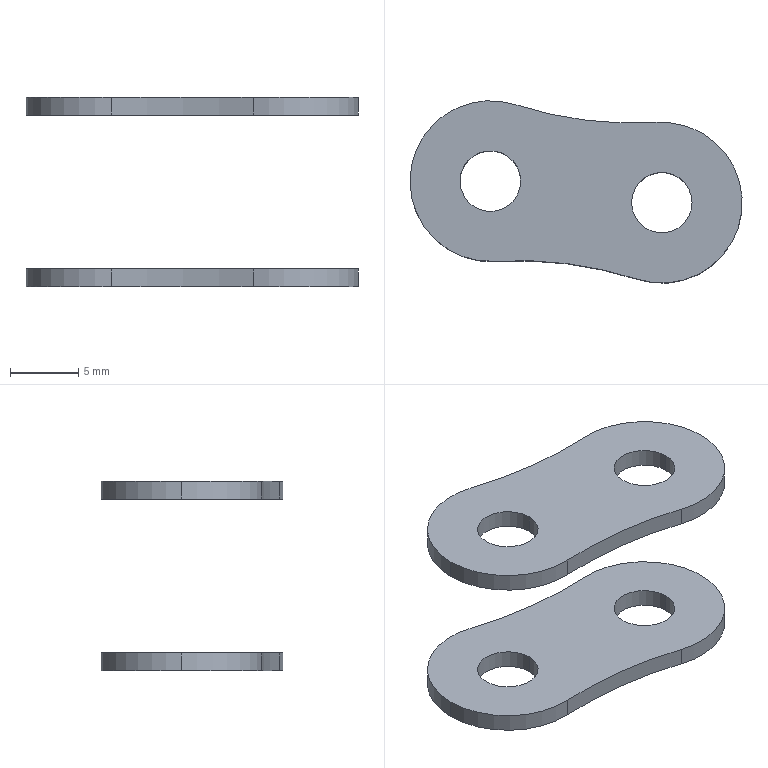Part | SolidWorks | features Boss 2, DeleteBody 1, Extrusion 1, MirrorSolid 1 | 2 solids | 22 faces | box 24.41 x 13.399 x 13.92 mm | volume 574.494 mm3 | cylinder 18 | plane 4 | commonest cylinder face diameters 4.45 x8 11.81 x6 57.066 x4
STEP:
#1=CARTESIAN_POINT('',(16.725,-1.589,6.96));
#2=VERTEX_POINT('',#1);
#3=CARTESIAN_POINT('',(21.175,-1.589,6.96));
#4=VERTEX_POINT('',#3);
#5=CARTESIAN_POINT('',(18.95,-1.589,6.96));
#6=DIRECTION('',(0.,0.,1.));
#7=DIRECTION('',(1.,0.,0.));
#8=AXIS2_PLACEMENT_3D('',#5,#6,#7);
#9=CIRCLE('',#8,2.225);
#10=EDGE_CURVE('',#2,#4,#9,.T.);
#11=ORIENTED_EDGE('',*,*,#10,.T.);
#12=CARTESIAN_POINT('',(21.175,-1.589,5.65));
#13=VERTEX_POINT('',#12);
#14=CARTESIAN_POINT('',(21.175,-1.589,6.96));
#15=DIRECTION('',(0.,0.,-1.));
#16=VECTOR('',#15,1000.);
#17=LINE('',#14,#16);
#18=EDGE_CURVE('',#4,#13,#17,.T.);
#19=ORIENTED_EDGE('',*,*,#18,.T.);
#20=CARTESIAN_POINT('',(16.725,-1.589,5.65));
#21=VERTEX_POINT('',#20);
#22=CARTESIAN_POINT('',(18.95,-1.589,5.65));
#23=DIRECTION('',(0.,0.,1.));
#24=DIRECTION('',(1.,0.,0.));
#25=AXIS2_PLACEMENT_3D('',#22,#23,#24);
#26=CIRCLE('',#25,2.225);
#27=EDGE_CURVE('',#21,#13,#26,.T.);
#28=ORIENTED_EDGE('',*,*,#27,.F.);
#29=CARTESIAN_POINT('',(16.725,-1.589,6.96));
#30=DIRECTION('',(0.,0.,-1.));
#31=VECTOR('',#30,1000.);
#32=LINE('',#29,#31);
#33=EDGE_CURVE('',#2,#21,#32,.T.);
#34=ORIENTED_EDGE('',*,*,#33,.F.);
#35=EDGE_LOOP('',(#11,#19,#28,#34));
#36=FACE_OUTER_BOUND('',#35,.T.);
#37=CARTESIAN_POINT('',(18.95,-1.589,6.96));
#38=DIRECTION('',(0.,0.,-1.));
#39=DIRECTION('',(-1.,0.,0.));
#40=AXIS2_PLACEMENT_3D('',#37,#38,#39);
#41=CYLINDRICAL_SURFACE('',#40,2.225);
#42=ADVANCED_FACE('',(#36),#41,.F.);
#43=CARTESIAN_POINT('',(4.125,0.,6.96));
#44=VERTEX_POINT('',#43);
#45=CARTESIAN_POINT('',(8.575,0.,6.96));
#46=VERTEX_POINT('',#45);
#47=CARTESIAN_POINT('',(6.35,0.,6.96));
#48=DIRECTION('',(0.,0.,1.));
#49=DIRECTION('',(1.,0.,0.));
#50=AXIS2_PLACEMENT_3D('',#47,#48,#49);
#51=CIRCLE('',#50,2.225);
#52=EDGE_CURVE('',#44,#46,#51,.T.);
#53=ORIENTED_EDGE('',*,*,#52,.T.);
#54=CARTESIAN_POINT('',(8.575,0.,5.65));
#55=VERTEX_POINT('',#54);
#56=CARTESIAN_POINT('',(8.575,0.,6.96));
#57=DIRECTION('',(0.,0.,-1.));
#58=VECTOR('',#57,1000.);
#59=LINE('',#56,#58);
#60=EDGE_CURVE('',#46,#55,#59,.T.);
#61=ORIENTED_EDGE('',*,*,#60,.T.);
#62=CARTESIAN_POINT('',(4.125,0.,5.65));
#63=VERTEX_POINT('',#62);
#64=CARTESIAN_POINT('',(6.35,0.,5.65));
#65=DIRECTION('',(0.,0.,1.));
#66=DIRECTION('',(1.,0.,0.));
#67=AXIS2_PLACEMENT_3D('',#64,#65,#66);
#68=CIRCLE('',#67,2.225);
#69=EDGE_CURVE('',#63,#55,#68,.T.);
#70=ORIENTED_EDGE('',*,*,#69,.F.);
#71=CARTESIAN_POINT('',(4.125,0.,6.96));
#72=DIRECTION('',(0.,0.,-1.));
#73=VECTOR('',#72,1000.);
#74=LINE('',#71,#73);
#75=EDGE_CURVE('',#44,#63,#74,.T.);
#76=ORIENTED_EDGE('',*,*,#75,.F.);
#77=EDGE_LOOP('',(#53,#61,#70,#76));
#78=FACE_OUTER_BOUND('',#77,.T.);
#79=CARTESIAN_POINT('',(6.35,0.,6.96));
#80=DIRECTION('',(0.,0.,-1.));
#81=DIRECTION('',(-1.,0.,0.));
#82=AXIS2_PLACEMENT_3D('',#79,#80,#81);
#83=CYLINDRICAL_SURFACE('',#82,2.225);
#84=ADVANCED_FACE('',(#78),#83,.F.);
#85=CARTESIAN_POINT('',(0.445,0.,6.96));
#86=VERTEX_POINT('',#85);
#87=CARTESIAN_POINT('',(6.704,-5.894,6.96));
#88=VERTEX_POINT('',#87);
#89=CARTESIAN_POINT('',(6.35,0.,6.96));
#90=DIRECTION('',(0.,0.,1.));
#91=DIRECTION('',(1.,0.,0.));
#92=AXIS2_PLACEMENT_3D('',#89,#90,#91);
#93=CIRCLE('',#92,5.905);
#94=EDGE_CURVE('',#86,#88,#93,.T.);
#95=ORIENTED_EDGE('',*,*,#94,.F.);
#96=CARTESIAN_POINT('',(0.445,0.,5.65));
#97=VERTEX_POINT('',#96);
#98=CARTESIAN_POINT('',(0.445,0.,6.96));
#99=DIRECTION('',(0.,0.,-1.));
#100=VECTOR('',#99,1000.);
#101=LINE('',#98,#100);
#102=EDGE_CURVE('',#86,#97,#101,.T.);
#103=ORIENTED_EDGE('',*,*,#102,.T.);
#104=CARTESIAN_POINT('',(6.704,-5.894,5.65));
#105=VERTEX_POINT('',#104);
#106=CARTESIAN_POINT('',(6.35,0.,5.65));
#107=DIRECTION('',(0.,0.,1.));
#108=DIRECTION('',(1.,0.,0.));
#109=AXIS2_PLACEMENT_3D('',#106,#107,#108);
#110=CIRCLE('',#109,5.905);
#111=EDGE_CURVE('',#97,#105,#110,.T.);
#112=ORIENTED_EDGE('',*,*,#111,.T.);
#113=CARTESIAN_POINT('',(6.704,-5.894,6.96));
#114=DIRECTION('',(0.,0.,-1.));
#115=VECTOR('',#114,1000.);
#116=LINE('',#113,#115);
#117=EDGE_CURVE('',#88,#105,#116,.T.);
#118=ORIENTED_EDGE('',*,*,#117,.F.);
#119=EDGE_LOOP('',(#95,#103,#112,#118));
#120=FACE_OUTER_BOUND('',#119,.T.);
#121=CARTESIAN_POINT('',(6.35,0.,6.96));
#122=DIRECTION('',(0.,0.,-1.));
#123=DIRECTION('',(-1.,0.,0.));
#124=AXIS2_PLACEMENT_3D('',#121,#122,#123);
#125=CYLINDRICAL_SURFACE('',#124,5.905);
#126=ADVANCED_FACE('',(#120),#125,.T.);
#127=ORIENTED_EDGE('',*,*,#52,.F.);
#128=CARTESIAN_POINT('',(6.35,0.,6.96));
#129=DIRECTION('',(0.,0.,1.));
#130=DIRECTION('',(1.,0.,0.));
#131=AXIS2_PLACEMENT_3D('',#128,#129,#130);
#132=CIRCLE('',#131,2.225);
#133=EDGE_CURVE('',#46,#44,#132,.T.);
#134=ORIENTED_EDGE('',*,*,#133,.F.);
#135=EDGE_LOOP('',(#127,#134));
#136=FACE_BOUND('',#135,.T.);
#137=CARTESIAN_POINT('',(18.596,4.306,6.96));
#138=VERTEX_POINT('',#137);
#139=CARTESIAN_POINT('',(8.156,5.622,6.96));
#140=VERTEX_POINT('',#139);
#141=CARTESIAN_POINT('',(16.884,32.787,6.96));
#142=DIRECTION('',(0.,0.,-1.));
#143=DIRECTION('',(1.,0.,0.));
#144=AXIS2_PLACEMENT_3D('',#141,#142,#143);
#145=CIRCLE('',#144,28.533);
#146=EDGE_CURVE('',#138,#140,#145,.T.);
#147=ORIENTED_EDGE('',*,*,#146,.T.);
#148=CARTESIAN_POINT('',(6.35,0.,6.96));
#149=DIRECTION('',(0.,0.,1.));
#150=DIRECTION('',(1.,0.,0.));
#151=AXIS2_PLACEMENT_3D('',#148,#149,#150);
#152=CIRCLE('',#151,5.905);
#153=EDGE_CURVE('',#140,#86,#152,.T.);
#154=ORIENTED_EDGE('',*,*,#153,.T.);
#155=ORIENTED_EDGE('',*,*,#94,.T.);
#156=CARTESIAN_POINT('',(17.144,-7.211,6.96));
#157=VERTEX_POINT('',#156);
#158=CARTESIAN_POINT('',(8.416,-34.376,6.96));
#159=DIRECTION('',(0.,0.,-1.));
#160=DIRECTION('',(-1.,0.,0.));
#161=AXIS2_PLACEMENT_3D('',#158,#159,#160);
#162=CIRCLE('',#161,28.533);
#163=EDGE_CURVE('',#88,#157,#162,.T.);
#164=ORIENTED_EDGE('',*,*,#163,.T.);
#165=CARTESIAN_POINT('',(18.95,-1.589,6.96));
#166=DIRECTION('',(0.,0.,1.));
#167=DIRECTION('',(1.,0.,0.));
#168=AXIS2_PLACEMENT_3D('',#165,#166,#167);
#169=CIRCLE('',#168,5.905);
#170=EDGE_CURVE('',#157,#138,#169,.T.);
#171=ORIENTED_EDGE('',*,*,#170,.T.);
#172=EDGE_LOOP('',(#147,#154,#155,#164,#171));
#173=FACE_OUTER_BOUND('',#172,.T.);
#174=ORIENTED_EDGE('',*,*,#10,.F.);
#175=CARTESIAN_POINT('',(18.95,-1.589,6.96));
#176=DIRECTION('',(0.,0.,1.));
#177=DIRECTION('',(1.,0.,0.));
#178=AXIS2_PLACEMENT_3D('',#175,#176,#177);
#179=CIRCLE('',#178,2.225);
#180=EDGE_CURVE('',#4,#2,#179,.T.);
#181=ORIENTED_EDGE('',*,*,#180,.F.);
#182=EDGE_LOOP('',(#174,#181));
#183=FACE_BOUND('',#182,.T.);
#184=CARTESIAN_POINT('',(17.917,15.599,6.96));
#185=DIRECTION('',(0.,0.,1.));
#186=DIRECTION('',(1.,0.,0.));
#187=AXIS2_PLACEMENT_3D('',#184,#185,#186);
#188=PLANE('',#187);
#189=ADVANCED_FACE('',(#136,#173,#183),#188,.T.);
#190=CARTESIAN_POINT('',(18.596,4.306,5.65));
#191=VERTEX_POINT('',#190);
#192=CARTESIAN_POINT('',(8.156,5.622,5.65));
#193=VERTEX_POINT('',#192);
#194=CARTESIAN_POINT('',(16.884,32.787,5.65));
#195=DIRECTION('',(0.,0.,-1.));
#196=DIRECTION('',(1.,0.,0.));
#197=AXIS2_PLACEMENT_3D('',#194,#195,#196);
#198=CIRCLE('',#197,28.533);
#199=EDGE_CURVE('',#191,#193,#198,.T.);
#200=ORIENTED_EDGE('',*,*,#199,.F.);
#201=CARTESIAN_POINT('',(17.144,-7.211,5.65));
#202=VERTEX_POINT('',#201);
#203=CARTESIAN_POINT('',(18.95,-1.589,5.65));
#204=DIRECTION('',(0.,0.,1.));
#205=DIRECTION('',(1.,0.,0.));
#206=AXIS2_PLACEMENT_3D('',#203,#204,#205);
#207=CIRCLE('',#206,5.905);
#208=EDGE_CURVE('',#202,#191,#207,.T.);
#209=ORIENTED_EDGE('',*,*,#208,.F.);
#210=CARTESIAN_POINT('',(8.416,-34.376,5.65));
#211=DIRECTION('',(0.,0.,-1.));
#212=DIRECTION('',(-1.,0.,0.));
#213=AXIS2_PLACEMENT_3D('',#210,#211,#212);
#214=CIRCLE('',#213,28.533);
#215=EDGE_CURVE('',#105,#202,#214,.T.);
#216=ORIENTED_EDGE('',*,*,#215,.F.);
#217=ORIENTED_EDGE('',*,*,#111,.F.);
#218=CARTESIAN_POINT('',(6.35,0.,5.65));
#219=DIRECTION('',(0.,0.,1.));
#220=DIRECTION('',(1.,0.,0.));
#221=AXIS2_PLACEMENT_3D('',#218,#219,#220);
#222=CIRCLE('',#221,5.905);
#223=EDGE_CURVE('',#193,#97,#222,.T.);
#224=ORIENTED_EDGE('',*,*,#223,.F.);
#225=EDGE_LOOP('',(#200,#209,#216,#217,#224));
#226=FACE_OUTER_BOUND('',#225,.T.);
#227=ORIENTED_EDGE('',*,*,#69,.T.);
#228=CARTESIAN_POINT('',(6.35,0.,5.65));
#229=DIRECTION('',(0.,0.,1.));
#230=DIRECTION('',(1.,0.,0.));
#231=AXIS2_PLACEMENT_3D('',#228,#229,#230);
#232=CIRCLE('',#231,2.225);
#233=EDGE_CURVE('',#55,#63,#232,.T.);
#234=ORIENTED_EDGE('',*,*,#233,.T.);
#235=EDGE_LOOP('',(#227,#234));
#236=FACE_BOUND('',#235,.T.);
#237=ORIENTED_EDGE('',*,*,#27,.T.);
#238=CARTESIAN_POINT('',(18.95,-1.589,5.65));
#239=DIRECTION('',(0.,0.,1.));
#240=DIRECTION('',(1.,0.,0.));
#241=AXIS2_PLACEMENT_3D('',#238,#239,#240);
#242=CIRCLE('',#241,2.225);
#243=EDGE_CURVE('',#13,#21,#242,.T.);
#244=ORIENTED_EDGE('',*,*,#243,.T.);
#245=EDGE_LOOP('',(#237,#244));
#246=FACE_BOUND('',#245,.T.);
#247=CARTESIAN_POINT('',(17.917,15.599,5.65));
#248=DIRECTION('',(0.,0.,1.));
#249=DIRECTION('',(1.,0.,0.));
#250=AXIS2_PLACEMENT_3D('',#247,#248,#249);
#251=PLANE('',#250);
#252=ADVANCED_FACE('',(#226,#236,#246),#251,.F.);
#253=ORIENTED_EDGE('',*,*,#199,.T.);
#254=CARTESIAN_POINT('',(8.156,5.622,6.96));
#255=DIRECTION('',(0.,0.,-1.));
#256=VECTOR('',#255,1000.);
#257=LINE('',#254,#256);
#258=EDGE_CURVE('',#140,#193,#257,.T.);
#259=ORIENTED_EDGE('',*,*,#258,.F.);
#260=ORIENTED_EDGE('',*,*,#146,.F.);
#261=CARTESIAN_POINT('',(18.596,4.306,6.96));
#262=DIRECTION('',(0.,0.,-1.));
#263=VECTOR('',#262,1000.);
#264=LINE('',#261,#263);
#265=EDGE_CURVE('',#138,#191,#264,.T.);
#266=ORIENTED_EDGE('',*,*,#265,.T.);
#267=EDGE_LOOP('',(#253,#259,#260,#266));
#268=FACE_OUTER_BOUND('',#267,.T.);
#269=CARTESIAN_POINT('',(16.884,32.787,6.96));
#270=DIRECTION('',(0.,0.,-1.));
#271=DIRECTION('',(-1.,0.,0.));
#272=AXIS2_PLACEMENT_3D('',#269,#270,#271);
#273=CYLINDRICAL_SURFACE('',#272,28.533);
#274=ADVANCED_FACE('',(#268),#273,.F.);
#275=ORIENTED_EDGE('',*,*,#102,.F.);
#276=ORIENTED_EDGE('',*,*,#153,.F.);
#277=ORIENTED_EDGE('',*,*,#258,.T.);
#278=ORIENTED_EDGE('',*,*,#223,.T.);
#279=EDGE_LOOP('',(#275,#276,#277,#278));
#280=FACE_OUTER_BOUND('',#279,.T.);
#281=CARTESIAN_POINT('',(6.35,0.,6.96));
#282=DIRECTION('',(0.,0.,-1.));
#283=DIRECTION('',(-1.,0.,0.));
#284=AXIS2_PLACEMENT_3D('',#281,#282,#283);
#285=CYLINDRICAL_SURFACE('',#284,5.905);
#286=ADVANCED_FACE('',(#280),#285,.T.);
#287=ORIENTED_EDGE('',*,*,#215,.T.);
#288=CARTESIAN_POINT('',(17.144,-7.211,6.96));
#289=DIRECTION('',(0.,0.,-1.));
#290=VECTOR('',#289,1000.);
#291=LINE('',#288,#290);
#292=EDGE_CURVE('',#157,#202,#291,.T.);
#293=ORIENTED_EDGE('',*,*,#292,.F.);
#294=ORIENTED_EDGE('',*,*,#163,.F.);
#295=ORIENTED_EDGE('',*,*,#117,.T.);
#296=EDGE_LOOP('',(#287,#293,#294,#295));
#297=FACE_OUTER_BOUND('',#296,.T.);
#298=CARTESIAN_POINT('',(8.416,-34.376,6.96));
#299=DIRECTION('',(0.,0.,-1.));
#300=DIRECTION('',(-1.,0.,0.));
#301=AXIS2_PLACEMENT_3D('',#298,#299,#300);
#302=CYLINDRICAL_SURFACE('',#301,28.533);
#303=ADVANCED_FACE('',(#297),#302,.F.);
#304=ORIENTED_EDGE('',*,*,#208,.T.);
#305=ORIENTED_EDGE('',*,*,#265,.F.);
#306=ORIENTED_EDGE('',*,*,#170,.F.);
#307=ORIENTED_EDGE('',*,*,#292,.T.);
#308=EDGE_LOOP('',(#304,#305,#306,#307));
#309=FACE_OUTER_BOUND('',#308,.T.);
#310=CARTESIAN_POINT('',(18.95,-1.589,6.96));
#311=DIRECTION('',(0.,0.,-1.));
#312=DIRECTION('',(-1.,0.,0.));
#313=AXIS2_PLACEMENT_3D('',#310,#311,#312);
#314=CYLINDRICAL_SURFACE('',#313,5.905);
#315=ADVANCED_FACE('',(#309),#314,.T.);
#316=ORIENTED_EDGE('',*,*,#60,.F.);
#317=ORIENTED_EDGE('',*,*,#133,.T.);
#318=ORIENTED_EDGE('',*,*,#75,.T.);
#319=ORIENTED_EDGE('',*,*,#233,.F.);
#320=EDGE_LOOP('',(#316,#317,#318,#319));
#321=FACE_OUTER_BOUND('',#320,.T.);
#322=CARTESIAN_POINT('',(6.35,0.,6.96));
#323=DIRECTION('',(0.,0.,-1.));
#324=DIRECTION('',(-1.,0.,0.));
#325=AXIS2_PLACEMENT_3D('',#322,#323,#324);
#326=CYLINDRICAL_SURFACE('',#325,2.225);
#327=ADVANCED_FACE('',(#321),#326,.F.);
#328=ORIENTED_EDGE('',*,*,#18,.F.);
#329=ORIENTED_EDGE('',*,*,#180,.T.);
#330=ORIENTED_EDGE('',*,*,#33,.T.);
#331=ORIENTED_EDGE('',*,*,#243,.F.);
#332=EDGE_LOOP('',(#328,#329,#330,#331));
#333=FACE_OUTER_BOUND('',#332,.T.);
#334=CARTESIAN_POINT('',(18.95,-1.589,6.96));
#335=DIRECTION('',(0.,0.,-1.));
#336=DIRECTION('',(-1.,0.,0.));
#337=AXIS2_PLACEMENT_3D('',#334,#335,#336);
#338=CYLINDRICAL_SURFACE('',#337,2.225);
#339=ADVANCED_FACE('',(#333),#338,.F.);
#340=CLOSED_SHELL('',(#42,#84,#126,#189,#252,#274,#286,#303,#315,#327,#339));
#341=MANIFOLD_SOLID_BREP('',#340);
#342=CARTESIAN_POINT('',(21.175,-1.589,-6.96));
#343=VERTEX_POINT('',#342);
#344=CARTESIAN_POINT('',(16.725,-1.589,-6.96));
#345=VERTEX_POINT('',#344);
#346=CARTESIAN_POINT('',(18.95,-1.589,-6.96));
#347=DIRECTION('',(0.,0.,1.));
#348=DIRECTION('',(1.,0.,0.));
#349=AXIS2_PLACEMENT_3D('',#346,#347,#348);
#350=CIRCLE('',#349,2.225);
#351=EDGE_CURVE('',#343,#345,#350,.T.);
#352=ORIENTED_EDGE('',*,*,#351,.F.);
#353=CARTESIAN_POINT('',(21.175,-1.589,-5.65));
#354=VERTEX_POINT('',#353);
#355=CARTESIAN_POINT('',(21.175,-1.589,-6.96));
#356=DIRECTION('',(0.,0.,1.));
#357=VECTOR('',#356,1000.);
#358=LINE('',#355,#357);
#359=EDGE_CURVE('',#343,#354,#358,.T.);
#360=ORIENTED_EDGE('',*,*,#359,.T.);
#361=CARTESIAN_POINT('',(16.725,-1.589,-5.65));
#362=VERTEX_POINT('',#361);
#363=CARTESIAN_POINT('',(18.95,-1.589,-5.65));
#364=DIRECTION('',(0.,0.,1.));
#365=DIRECTION('',(1.,0.,0.));
#366=AXIS2_PLACEMENT_3D('',#363,#364,#365);
#367=CIRCLE('',#366,2.225);
#368=EDGE_CURVE('',#354,#362,#367,.T.);
#369=ORIENTED_EDGE('',*,*,#368,.T.);
#370=CARTESIAN_POINT('',(16.725,-1.589,-6.96));
#371=DIRECTION('',(0.,0.,1.));
#372=VECTOR('',#371,1000.);
#373=LINE('',#370,#372);
#374=EDGE_CURVE('',#345,#362,#373,.T.);
#375=ORIENTED_EDGE('',*,*,#374,.F.);
#376=EDGE_LOOP('',(#352,#360,#369,#375));
#377=FACE_OUTER_BOUND('',#376,.T.);
#378=CARTESIAN_POINT('',(18.95,-1.589,-6.96));
#379=DIRECTION('',(0.,0.,1.));
#380=DIRECTION('',(-1.,0.,0.));
#381=AXIS2_PLACEMENT_3D('',#378,#379,#380);
#382=CYLINDRICAL_SURFACE('',#381,2.225);
#383=ADVANCED_FACE('',(#377),#382,.F.);
#384=CARTESIAN_POINT('',(8.575,0.,-6.96));
#385=VERTEX_POINT('',#384);
#386=CARTESIAN_POINT('',(4.125,0.,-6.96));
#387=VERTEX_POINT('',#386);
#388=CARTESIAN_POINT('',(6.35,0.,-6.96));
#389=DIRECTION('',(0.,0.,1.));
#390=DIRECTION('',(1.,0.,0.));
#391=AXIS2_PLACEMENT_3D('',#388,#389,#390);
#392=CIRCLE('',#391,2.225);
#393=EDGE_CURVE('',#385,#387,#392,.T.);
#394=ORIENTED_EDGE('',*,*,#393,.F.);
#395=CARTESIAN_POINT('',(8.575,0.,-5.65));
#396=VERTEX_POINT('',#395);
#397=CARTESIAN_POINT('',(8.575,0.,-6.96));
#398=DIRECTION('',(0.,0.,1.));
#399=VECTOR('',#398,1000.);
#400=LINE('',#397,#399);
#401=EDGE_CURVE('',#385,#396,#400,.T.);
#402=ORIENTED_EDGE('',*,*,#401,.T.);
#403=CARTESIAN_POINT('',(4.125,0.,-5.65));
#404=VERTEX_POINT('',#403);
#405=CARTESIAN_POINT('',(6.35,0.,-5.65));
#406=DIRECTION('',(0.,0.,1.));
#407=DIRECTION('',(1.,0.,0.));
#408=AXIS2_PLACEMENT_3D('',#405,#406,#407);
#409=CIRCLE('',#408,2.225);
#410=EDGE_CURVE('',#396,#404,#409,.T.);
#411=ORIENTED_EDGE('',*,*,#410,.T.);
#412=CARTESIAN_POINT('',(4.125,0.,-6.96));
#413=DIRECTION('',(0.,0.,1.));
#414=VECTOR('',#413,1000.);
#415=LINE('',#412,#414);
#416=EDGE_CURVE('',#387,#404,#415,.T.);
#417=ORIENTED_EDGE('',*,*,#416,.F.);
#418=EDGE_LOOP('',(#394,#402,#411,#417));
#419=FACE_OUTER_BOUND('',#418,.T.);
#420=CARTESIAN_POINT('',(6.35,0.,-6.96));
#421=DIRECTION('',(0.,0.,1.));
#422=DIRECTION('',(-1.,0.,0.));
#423=AXIS2_PLACEMENT_3D('',#420,#421,#422);
#424=CYLINDRICAL_SURFACE('',#423,2.225);
#425=ADVANCED_FACE('',(#419),#424,.F.);
#426=CARTESIAN_POINT('',(8.156,5.622,-6.96));
#427=VERTEX_POINT('',#426);
#428=CARTESIAN_POINT('',(0.445,0.,-6.96));
#429=VERTEX_POINT('',#428);
#430=CARTESIAN_POINT('',(6.35,0.,-6.96));
#431=DIRECTION('',(0.,0.,1.));
#432=DIRECTION('',(1.,0.,0.));
#433=AXIS2_PLACEMENT_3D('',#430,#431,#432);
#434=CIRCLE('',#433,5.905);
#435=EDGE_CURVE('',#427,#429,#434,.T.);
#436=ORIENTED_EDGE('',*,*,#435,.T.);
#437=CARTESIAN_POINT('',(0.445,0.,-5.65));
#438=VERTEX_POINT('',#437);
#439=CARTESIAN_POINT('',(0.445,0.,-6.96));
#440=DIRECTION('',(0.,0.,1.));
#441=VECTOR('',#440,1000.);
#442=LINE('',#439,#441);
#443=EDGE_CURVE('',#429,#438,#442,.T.);
#444=ORIENTED_EDGE('',*,*,#443,.T.);
#445=CARTESIAN_POINT('',(8.156,5.622,-5.65));
#446=VERTEX_POINT('',#445);
#447=CARTESIAN_POINT('',(6.35,0.,-5.65));
#448=DIRECTION('',(0.,0.,1.));
#449=DIRECTION('',(1.,0.,0.));
#450=AXIS2_PLACEMENT_3D('',#447,#448,#449);
#451=CIRCLE('',#450,5.905);
#452=EDGE_CURVE('',#446,#438,#451,.T.);
#453=ORIENTED_EDGE('',*,*,#452,.F.);
#454=CARTESIAN_POINT('',(8.156,5.622,-6.96));
#455=DIRECTION('',(0.,0.,1.));
#456=VECTOR('',#455,1000.);
#457=LINE('',#454,#456);
#458=EDGE_CURVE('',#427,#446,#457,.T.);
#459=ORIENTED_EDGE('',*,*,#458,.F.);
#460=EDGE_LOOP('',(#436,#444,#453,#459));
#461=FACE_OUTER_BOUND('',#460,.T.);
#462=CARTESIAN_POINT('',(6.35,0.,-6.96));
#463=DIRECTION('',(0.,0.,1.));
#464=DIRECTION('',(-1.,0.,0.));
#465=AXIS2_PLACEMENT_3D('',#462,#463,#464);
#466=CYLINDRICAL_SURFACE('',#465,5.905);
#467=ADVANCED_FACE('',(#461),#466,.T.);
#468=CARTESIAN_POINT('',(6.35,0.,-6.96));
#469=DIRECTION('',(0.,0.,1.));
#470=DIRECTION('',(1.,0.,0.));
#471=AXIS2_PLACEMENT_3D('',#468,#469,#470);
#472=CIRCLE('',#471,2.225);
#473=EDGE_CURVE('',#387,#385,#472,.T.);
#474=ORIENTED_EDGE('',*,*,#473,.T.);
#475=ORIENTED_EDGE('',*,*,#393,.T.);
#476=EDGE_LOOP('',(#474,#475));
#477=FACE_BOUND('',#476,.T.);
#478=CARTESIAN_POINT('',(18.596,4.306,-6.96));
#479=VERTEX_POINT('',#478);
#480=CARTESIAN_POINT('',(16.884,32.787,-6.96));
#481=DIRECTION('',(0.,0.,-1.));
#482=DIRECTION('',(1.,0.,0.));
#483=AXIS2_PLACEMENT_3D('',#480,#481,#482);
#484=CIRCLE('',#483,28.533);
#485=EDGE_CURVE('',#479,#427,#484,.T.);
#486=ORIENTED_EDGE('',*,*,#485,.F.);
#487=CARTESIAN_POINT('',(17.144,-7.211,-6.96));
#488=VERTEX_POINT('',#487);
#489=CARTESIAN_POINT('',(18.95,-1.589,-6.96));
#490=DIRECTION('',(0.,0.,1.));
#491=DIRECTION('',(1.,0.,0.));
#492=AXIS2_PLACEMENT_3D('',#489,#490,#491);
#493=CIRCLE('',#492,5.905);
#494=EDGE_CURVE('',#488,#479,#493,.T.);
#495=ORIENTED_EDGE('',*,*,#494,.F.);
#496=CARTESIAN_POINT('',(6.704,-5.894,-6.96));
#497=VERTEX_POINT('',#496);
#498=CARTESIAN_POINT('',(8.416,-34.376,-6.96));
#499=DIRECTION('',(0.,0.,-1.));
#500=DIRECTION('',(-1.,0.,0.));
#501=AXIS2_PLACEMENT_3D('',#498,#499,#500);
#502=CIRCLE('',#501,28.533);
#503=EDGE_CURVE('',#497,#488,#502,.T.);
#504=ORIENTED_EDGE('',*,*,#503,.F.);
#505=CARTESIAN_POINT('',(6.35,0.,-6.96));
#506=DIRECTION('',(0.,0.,1.));
#507=DIRECTION('',(1.,0.,0.));
#508=AXIS2_PLACEMENT_3D('',#505,#506,#507);
#509=CIRCLE('',#508,5.905);
#510=EDGE_CURVE('',#429,#497,#509,.T.);
#511=ORIENTED_EDGE('',*,*,#510,.F.);
#512=ORIENTED_EDGE('',*,*,#435,.F.);
#513=EDGE_LOOP('',(#486,#495,#504,#511,#512));
#514=FACE_OUTER_BOUND('',#513,.T.);
#515=CARTESIAN_POINT('',(18.95,-1.589,-6.96));
#516=DIRECTION('',(0.,0.,1.));
#517=DIRECTION('',(1.,0.,0.));
#518=AXIS2_PLACEMENT_3D('',#515,#516,#517);
#519=CIRCLE('',#518,2.225);
#520=EDGE_CURVE('',#345,#343,#519,.T.);
#521=ORIENTED_EDGE('',*,*,#520,.T.);
#522=ORIENTED_EDGE('',*,*,#351,.T.);
#523=EDGE_LOOP('',(#521,#522));
#524=FACE_BOUND('',#523,.T.);
#525=CARTESIAN_POINT('',(17.917,15.599,-6.96));
#526=DIRECTION('',(0.,0.,-1.));
#527=DIRECTION('',(1.,0.,0.));
#528=AXIS2_PLACEMENT_3D('',#525,#526,#527);
#529=PLANE('',#528);
#530=ADVANCED_FACE('',(#477,#514,#524),#529,.T.);
#531=CARTESIAN_POINT('',(18.596,4.306,-5.65));
#532=VERTEX_POINT('',#531);
#533=CARTESIAN_POINT('',(16.884,32.787,-5.65));
#534=DIRECTION('',(0.,0.,-1.));
#535=DIRECTION('',(1.,0.,0.));
#536=AXIS2_PLACEMENT_3D('',#533,#534,#535);
#537=CIRCLE('',#536,28.533);
#538=EDGE_CURVE('',#532,#446,#537,.T.);
#539=ORIENTED_EDGE('',*,*,#538,.T.);
#540=ORIENTED_EDGE('',*,*,#452,.T.);
#541=CARTESIAN_POINT('',(6.704,-5.894,-5.65));
#542=VERTEX_POINT('',#541);
#543=CARTESIAN_POINT('',(6.35,0.,-5.65));
#544=DIRECTION('',(0.,0.,1.));
#545=DIRECTION('',(1.,0.,0.));
#546=AXIS2_PLACEMENT_3D('',#543,#544,#545);
#547=CIRCLE('',#546,5.905);
#548=EDGE_CURVE('',#438,#542,#547,.T.);
#549=ORIENTED_EDGE('',*,*,#548,.T.);
#550=CARTESIAN_POINT('',(17.144,-7.211,-5.65));
#551=VERTEX_POINT('',#550);
#552=CARTESIAN_POINT('',(8.416,-34.376,-5.65));
#553=DIRECTION('',(0.,0.,-1.));
#554=DIRECTION('',(-1.,0.,0.));
#555=AXIS2_PLACEMENT_3D('',#552,#553,#554);
#556=CIRCLE('',#555,28.533);
#557=EDGE_CURVE('',#542,#551,#556,.T.);
#558=ORIENTED_EDGE('',*,*,#557,.T.);
#559=CARTESIAN_POINT('',(18.95,-1.589,-5.65));
#560=DIRECTION('',(0.,0.,1.));
#561=DIRECTION('',(1.,0.,0.));
#562=AXIS2_PLACEMENT_3D('',#559,#560,#561);
#563=CIRCLE('',#562,5.905);
#564=EDGE_CURVE('',#551,#532,#563,.T.);
#565=ORIENTED_EDGE('',*,*,#564,.T.);
#566=EDGE_LOOP('',(#539,#540,#549,#558,#565));
#567=FACE_OUTER_BOUND('',#566,.T.);
#568=CARTESIAN_POINT('',(6.35,0.,-5.65));
#569=DIRECTION('',(0.,0.,1.));
#570=DIRECTION('',(1.,0.,0.));
#571=AXIS2_PLACEMENT_3D('',#568,#569,#570);
#572=CIRCLE('',#571,2.225);
#573=EDGE_CURVE('',#404,#396,#572,.T.);
#574=ORIENTED_EDGE('',*,*,#573,.F.);
#575=ORIENTED_EDGE('',*,*,#410,.F.);
#576=EDGE_LOOP('',(#574,#575));
#577=FACE_BOUND('',#576,.T.);
#578=CARTESIAN_POINT('',(18.95,-1.589,-5.65));
#579=DIRECTION('',(0.,0.,1.));
#580=DIRECTION('',(1.,0.,0.));
#581=AXIS2_PLACEMENT_3D('',#578,#579,#580);
#582=CIRCLE('',#581,2.225);
#583=EDGE_CURVE('',#362,#354,#582,.T.);
#584=ORIENTED_EDGE('',*,*,#583,.F.);
#585=ORIENTED_EDGE('',*,*,#368,.F.);
#586=EDGE_LOOP('',(#584,#585));
#587=FACE_BOUND('',#586,.T.);
#588=CARTESIAN_POINT('',(17.917,15.599,-5.65));
#589=DIRECTION('',(0.,0.,-1.));
#590=DIRECTION('',(1.,0.,0.));
#591=AXIS2_PLACEMENT_3D('',#588,#589,#590);
#592=PLANE('',#591);
#593=ADVANCED_FACE('',(#567,#577,#587),#592,.F.);
#594=ORIENTED_EDGE('',*,*,#538,.F.);
#595=CARTESIAN_POINT('',(18.596,4.306,-6.96));
#596=DIRECTION('',(0.,0.,1.));
#597=VECTOR('',#596,1000.);
#598=LINE('',#595,#597);
#599=EDGE_CURVE('',#479,#532,#598,.T.);
#600=ORIENTED_EDGE('',*,*,#599,.F.);
#601=ORIENTED_EDGE('',*,*,#485,.T.);
#602=ORIENTED_EDGE('',*,*,#458,.T.);
#603=EDGE_LOOP('',(#594,#600,#601,#602));
#604=FACE_OUTER_BOUND('',#603,.T.);
#605=CARTESIAN_POINT('',(16.884,32.787,-6.96));
#606=DIRECTION('',(0.,0.,1.));
#607=DIRECTION('',(-1.,0.,0.));
#608=AXIS2_PLACEMENT_3D('',#605,#606,#607);
#609=CYLINDRICAL_SURFACE('',#608,28.533);
#610=ADVANCED_FACE('',(#604),#609,.F.);
#611=ORIENTED_EDGE('',*,*,#443,.F.);
#612=ORIENTED_EDGE('',*,*,#510,.T.);
#613=CARTESIAN_POINT('',(6.704,-5.894,-6.96));
#614=DIRECTION('',(0.,0.,1.));
#615=VECTOR('',#614,1000.);
#616=LINE('',#613,#615);
#617=EDGE_CURVE('',#497,#542,#616,.T.);
#618=ORIENTED_EDGE('',*,*,#617,.T.);
#619=ORIENTED_EDGE('',*,*,#548,.F.);
#620=EDGE_LOOP('',(#611,#612,#618,#619));
#621=FACE_OUTER_BOUND('',#620,.T.);
#622=CARTESIAN_POINT('',(6.35,0.,-6.96));
#623=DIRECTION('',(0.,0.,1.));
#624=DIRECTION('',(-1.,0.,0.));
#625=AXIS2_PLACEMENT_3D('',#622,#623,#624);
#626=CYLINDRICAL_SURFACE('',#625,5.905);
#627=ADVANCED_FACE('',(#621),#626,.T.);
#628=ORIENTED_EDGE('',*,*,#557,.F.);
#629=ORIENTED_EDGE('',*,*,#617,.F.);
#630=ORIENTED_EDGE('',*,*,#503,.T.);
#631=CARTESIAN_POINT('',(17.144,-7.211,-6.96));
#632=DIRECTION('',(0.,0.,1.));
#633=VECTOR('',#632,1000.);
#634=LINE('',#631,#633);
#635=EDGE_CURVE('',#488,#551,#634,.T.);
#636=ORIENTED_EDGE('',*,*,#635,.T.);
#637=EDGE_LOOP('',(#628,#629,#630,#636));
#638=FACE_OUTER_BOUND('',#637,.T.);
#639=CARTESIAN_POINT('',(8.416,-34.376,-6.96));
#640=DIRECTION('',(0.,0.,1.));
#641=DIRECTION('',(-1.,0.,0.));
#642=AXIS2_PLACEMENT_3D('',#639,#640,#641);
#643=CYLINDRICAL_SURFACE('',#642,28.533);
#644=ADVANCED_FACE('',(#638),#643,.F.);
#645=ORIENTED_EDGE('',*,*,#564,.F.);
#646=ORIENTED_EDGE('',*,*,#635,.F.);
#647=ORIENTED_EDGE('',*,*,#494,.T.);
#648=ORIENTED_EDGE('',*,*,#599,.T.);
#649=EDGE_LOOP('',(#645,#646,#647,#648));
#650=FACE_OUTER_BOUND('',#649,.T.);
#651=CARTESIAN_POINT('',(18.95,-1.589,-6.96));
#652=DIRECTION('',(0.,0.,1.));
#653=DIRECTION('',(-1.,0.,0.));
#654=AXIS2_PLACEMENT_3D('',#651,#652,#653);
#655=CYLINDRICAL_SURFACE('',#654,5.905);
#656=ADVANCED_FACE('',(#650),#655,.T.);
#657=ORIENTED_EDGE('',*,*,#401,.F.);
#658=ORIENTED_EDGE('',*,*,#473,.F.);
#659=ORIENTED_EDGE('',*,*,#416,.T.);
#660=ORIENTED_EDGE('',*,*,#573,.T.);
#661=EDGE_LOOP('',(#657,#658,#659,#660));
#662=FACE_OUTER_BOUND('',#661,.T.);
#663=CARTESIAN_POINT('',(6.35,0.,-6.96));
#664=DIRECTION('',(0.,0.,1.));
#665=DIRECTION('',(-1.,0.,0.));
#666=AXIS2_PLACEMENT_3D('',#663,#664,#665);
#667=CYLINDRICAL_SURFACE('',#666,2.225);
#668=ADVANCED_FACE('',(#662),#667,.F.);
#669=ORIENTED_EDGE('',*,*,#359,.F.);
#670=ORIENTED_EDGE('',*,*,#520,.F.);
#671=ORIENTED_EDGE('',*,*,#374,.T.);
#672=ORIENTED_EDGE('',*,*,#583,.T.);
#673=EDGE_LOOP('',(#669,#670,#671,#672));
#674=FACE_OUTER_BOUND('',#673,.T.);
#675=CARTESIAN_POINT('',(18.95,-1.589,-6.96));
#676=DIRECTION('',(0.,0.,1.));
#677=DIRECTION('',(-1.,0.,0.));
#678=AXIS2_PLACEMENT_3D('',#675,#676,#677);
#679=CYLINDRICAL_SURFACE('',#678,2.225);
#680=ADVANCED_FACE('',(#674),#679,.F.);
#681=CLOSED_SHELL('',(#383,#425,#467,#530,#593,#610,#627,#644,#656,#668,#680));
#682=MANIFOLD_SOLID_BREP('',#681);
#683=CARTESIAN_POINT('',(0.,0.,0.));
#684=DIRECTION('',(0.,0.,1.));
#685=DIRECTION('',(1.,0.,0.));
#686=AXIS2_PLACEMENT_3D('',#683,#684,#685);
#687=(LENGTH_UNIT()NAMED_UNIT(*)SI_UNIT(.MILLI.,.METRE.));
#688=UNCERTAINTY_MEASURE_WITH_UNIT(LENGTH_MEASURE(0.00001),#687,'','');
#689=(NAMED_UNIT(*)PLANE_ANGLE_UNIT()SI_UNIT($,.RADIAN.));
#690=(NAMED_UNIT(*)SI_UNIT($,.STERADIAN.)SOLID_ANGLE_UNIT());
#691=(GEOMETRIC_REPRESENTATION_CONTEXT(3)GLOBAL_UNCERTAINTY_ASSIGNED_CONTEXT((#688))GLOBAL_UNIT_ASSIGNED_CONTEXT((#687,#689,#690))REPRESENTATION_CONTEXT('',''));
#692=ADVANCED_BREP_SHAPE_REPRESENTATION('',(#341,#682,#686),#691);